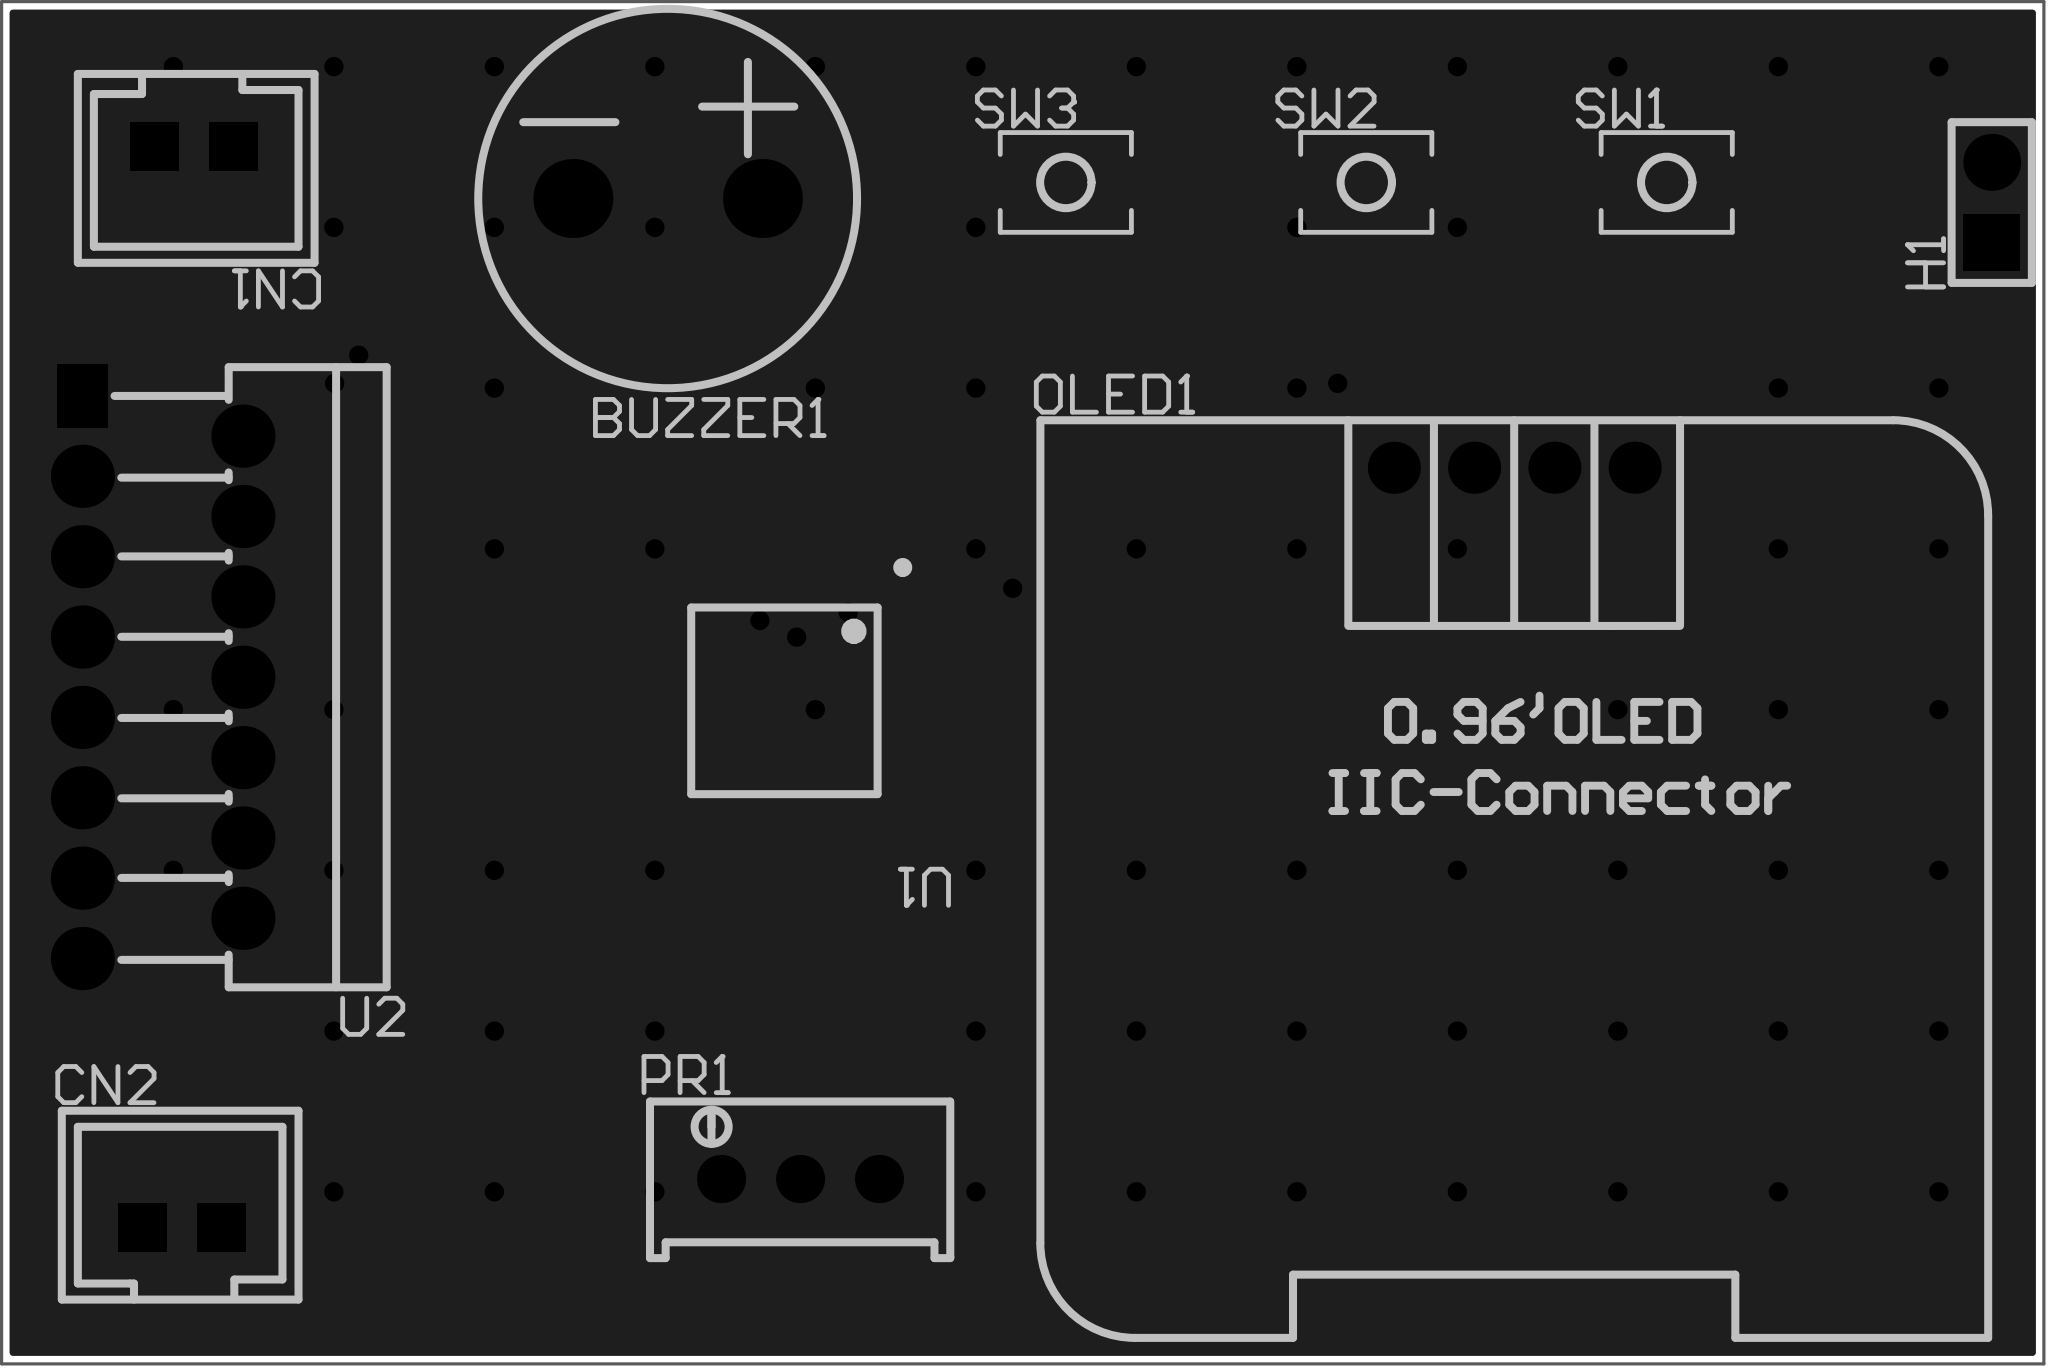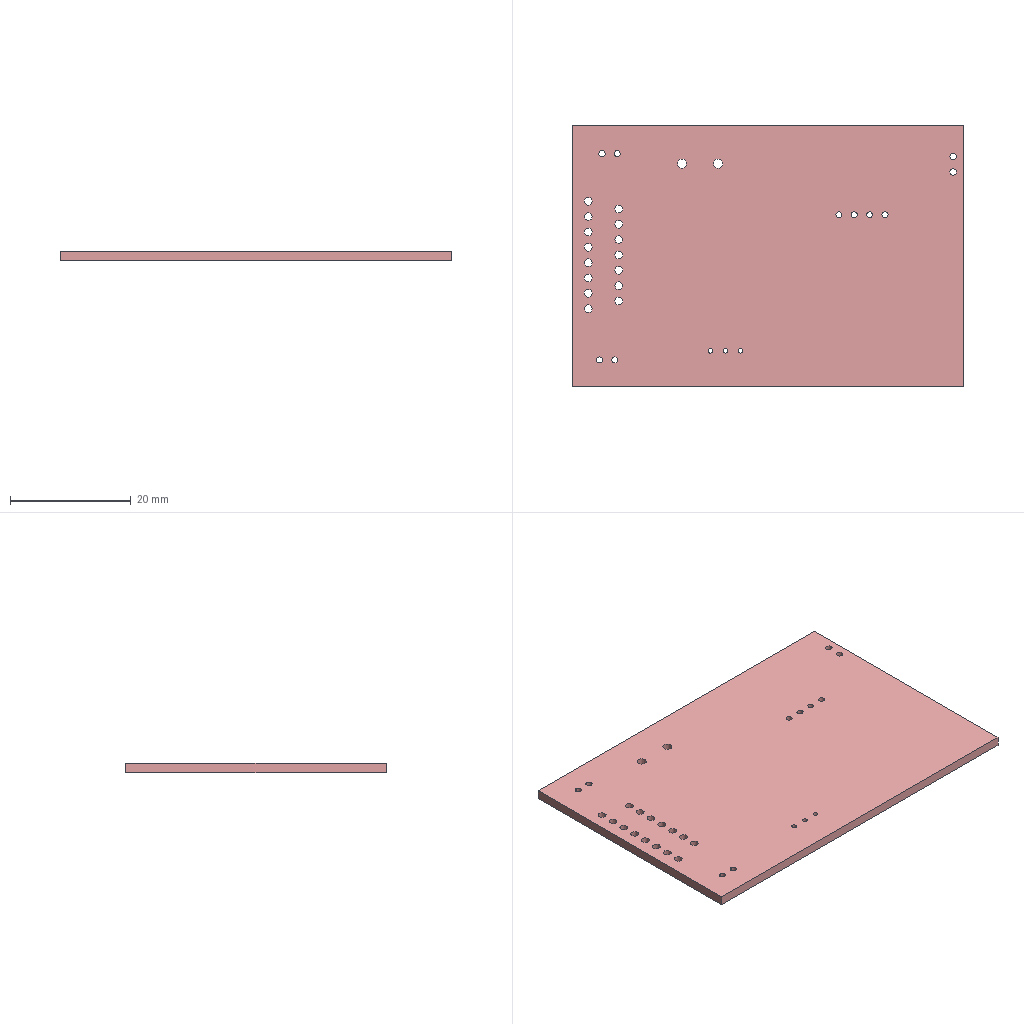Circuit board layout | Altium Designer | box 64.6 x 43.1 x 1.6 mm
Layer stack:
# Altium Designer layer stack of  (unit mm; dielectric type: 0 none, 1 core, 2 prepreg, 3 surface material)
index,name,kind,layer,copper_thickness_mm,dielectric_type,dielectric_thickness_mm,dielectric_material,dielectric_constant
0,Top Paste Mask Layer,other,,,,,,
1,Top Silkscreen Layer,other,,,,,,
2,Top Solder Mask Layer,dielectric,,,3,0.01,,3.3
3,Top Layer,copper,Top Layer,0.035,,,,
4,Dielectric1,dielectric,,,3,1.51,FR4,4.5
5,Bottom Layer,copper,Bottom Layer,0.035,,,,
6,Bottom Solder Mask Layer,dielectric,,,3,0.01,,3.3
7,Bottom Silkscreen Layer,other,,,,,,
8,Bottom Paste Mask Layer,other,,,,,,
# drill layer pairs: low layer,high layer
drill_pair,Top Layer,Bottom Layer
Part placement:
Designator,Comment,Layer,Footprint,Center-X(mm),Center-Y(mm),Rotation
BUZZER1,buzzer,TopLayer,BUZ-TH_BD12.0-P6.00-D0.9-RD,101.981,117.983,0
CN1,XH2.54-2PIN-直针,TopLayer,CONN-TH_XH2.54-2P,86.995,119.634,180
CN2,XH2.54-2PIN-直针,TopLayer,CONN-TH_XH2.54-2P,86.614,85.471,0
H1,,TopLayer,HDR-TH_2P-P2.54-V-M-1,143.891,117.856,90
OLED1,,TopLayer,0.96OLED_4P,128.778,109.474,0
PR1,10kΩ,TopLayer,R_3296,106.172,86.995,0
SW1,,TopLayer,Key_SMD_3x4x2,133.604,118.491,0
SW2,,TopLayer,Key_SMD_3x4x2,124.094,118.491,0
SW3,,TopLayer,Key_SMD_3x4x2,114.584,118.491,0
U1,ATMEGA328PB-AUR,TopLayer,TQFP-32_L7.0-W7.0-P0.80-LS9.0-BL,105.664,102.108,180
U2,L298N,TopLayer,MULTIWATT-15_L19.6-W5.0-P1.27-L,85.997,102.854,270
Pad and via stacks:
# Altium Designer via and pad stacks of  (unit mm). Each distinct definition once, with the count of objects using it.
# via: kind,start_layer,end_layer,hole_mm,diameter_mm,mode(0 simple;1 top-mid-bottom;2 full stack),diameter_per_layer,count,example_net
# pad: kind,layer,hole_mm,hole_type(0 round;1 square;2 slot),plating,top_size,top_shape(1 round;2 rect;3 octagon;9 rounded rect),mid_size,bottom_size,mode,footprint,size_per_layer,count,example
pad,Multi-Layer,1.5,0,plated,2.5x2.5,1,2.5x2.5,2.5x2.5,0,BUZ-TH_BD12.0-P6.00-D0.9-RD,,2,BUZZER1.1
pad,Multi-Layer,1,2,plated,1.524x1.524,2,1.524x1.524,1.524x1.524,0,CONN-TH_XH2.54-2P,,4,CN1.1
pad,Multi-Layer,1.1,0,plated,1.8x1.8,1,1.8x1.8,1.8x1.8,0,HDR-TH_2P-P2.54-V-M-1,,1,H1.2
pad,Multi-Layer,1.1,0,plated,1.8x1.8,2,1.8x1.8,1.8x1.8,0,HDR-TH_2P-P2.54-V-M-1,,1,H1.1
pad,Multi-Layer,1,0,plated,1.65x1.65,1,1.65x1.65,1.65x1.65,0,0.96OLED_4P,,4,OLED1.4
pad,Multi-Layer,0.762,0,plated,1.524x1.524,1,1.524x1.524,1.524x1.524,0,R_3296,,3,PR1.2
pad,Multi-Layer,1.3,0,plated,2x2,1,2x2,2x2,0,MULTIWATT-15_L19.6-W5.0-P1.27-L,,14,U2.15
pad,Multi-Layer,1.3,0,plated,2x1.6,2,2x1.6,2x1.6,0,MULTIWATT-15_L19.6-W5.0-P1.27-L,,1,U2.1
pad,Top Layer,0,0,plated,1.53x1.36,2,1.53x1.36,1.53x1.36,0,Key_SMD_3x4x2,,6,SW1.1
pad,Top Layer,0,0,plated,1.65x0.45,1,1.65x0.45,1.65x0.45,0,TQFP-32_L7.0-W7.0-P0.80-LS9.0-BL,,16,U1.32
pad,Top Layer,0,0,plated,0.45x1.65,1,0.45x1.65,0.45x1.65,0,TQFP-32_L7.0-W7.0-P0.80-LS9.0-BL,,16,U1.24
via,Top Layer,Bottom Layer,0.3048,0.61,0,,76,+5V
Copper pours:
name,layer,net,type(0 solid;1 hatched;2 none)
Bottom Layer-GND,Bottom Layer,GND,0
Top Layer-GND,Top Layer,GND,0